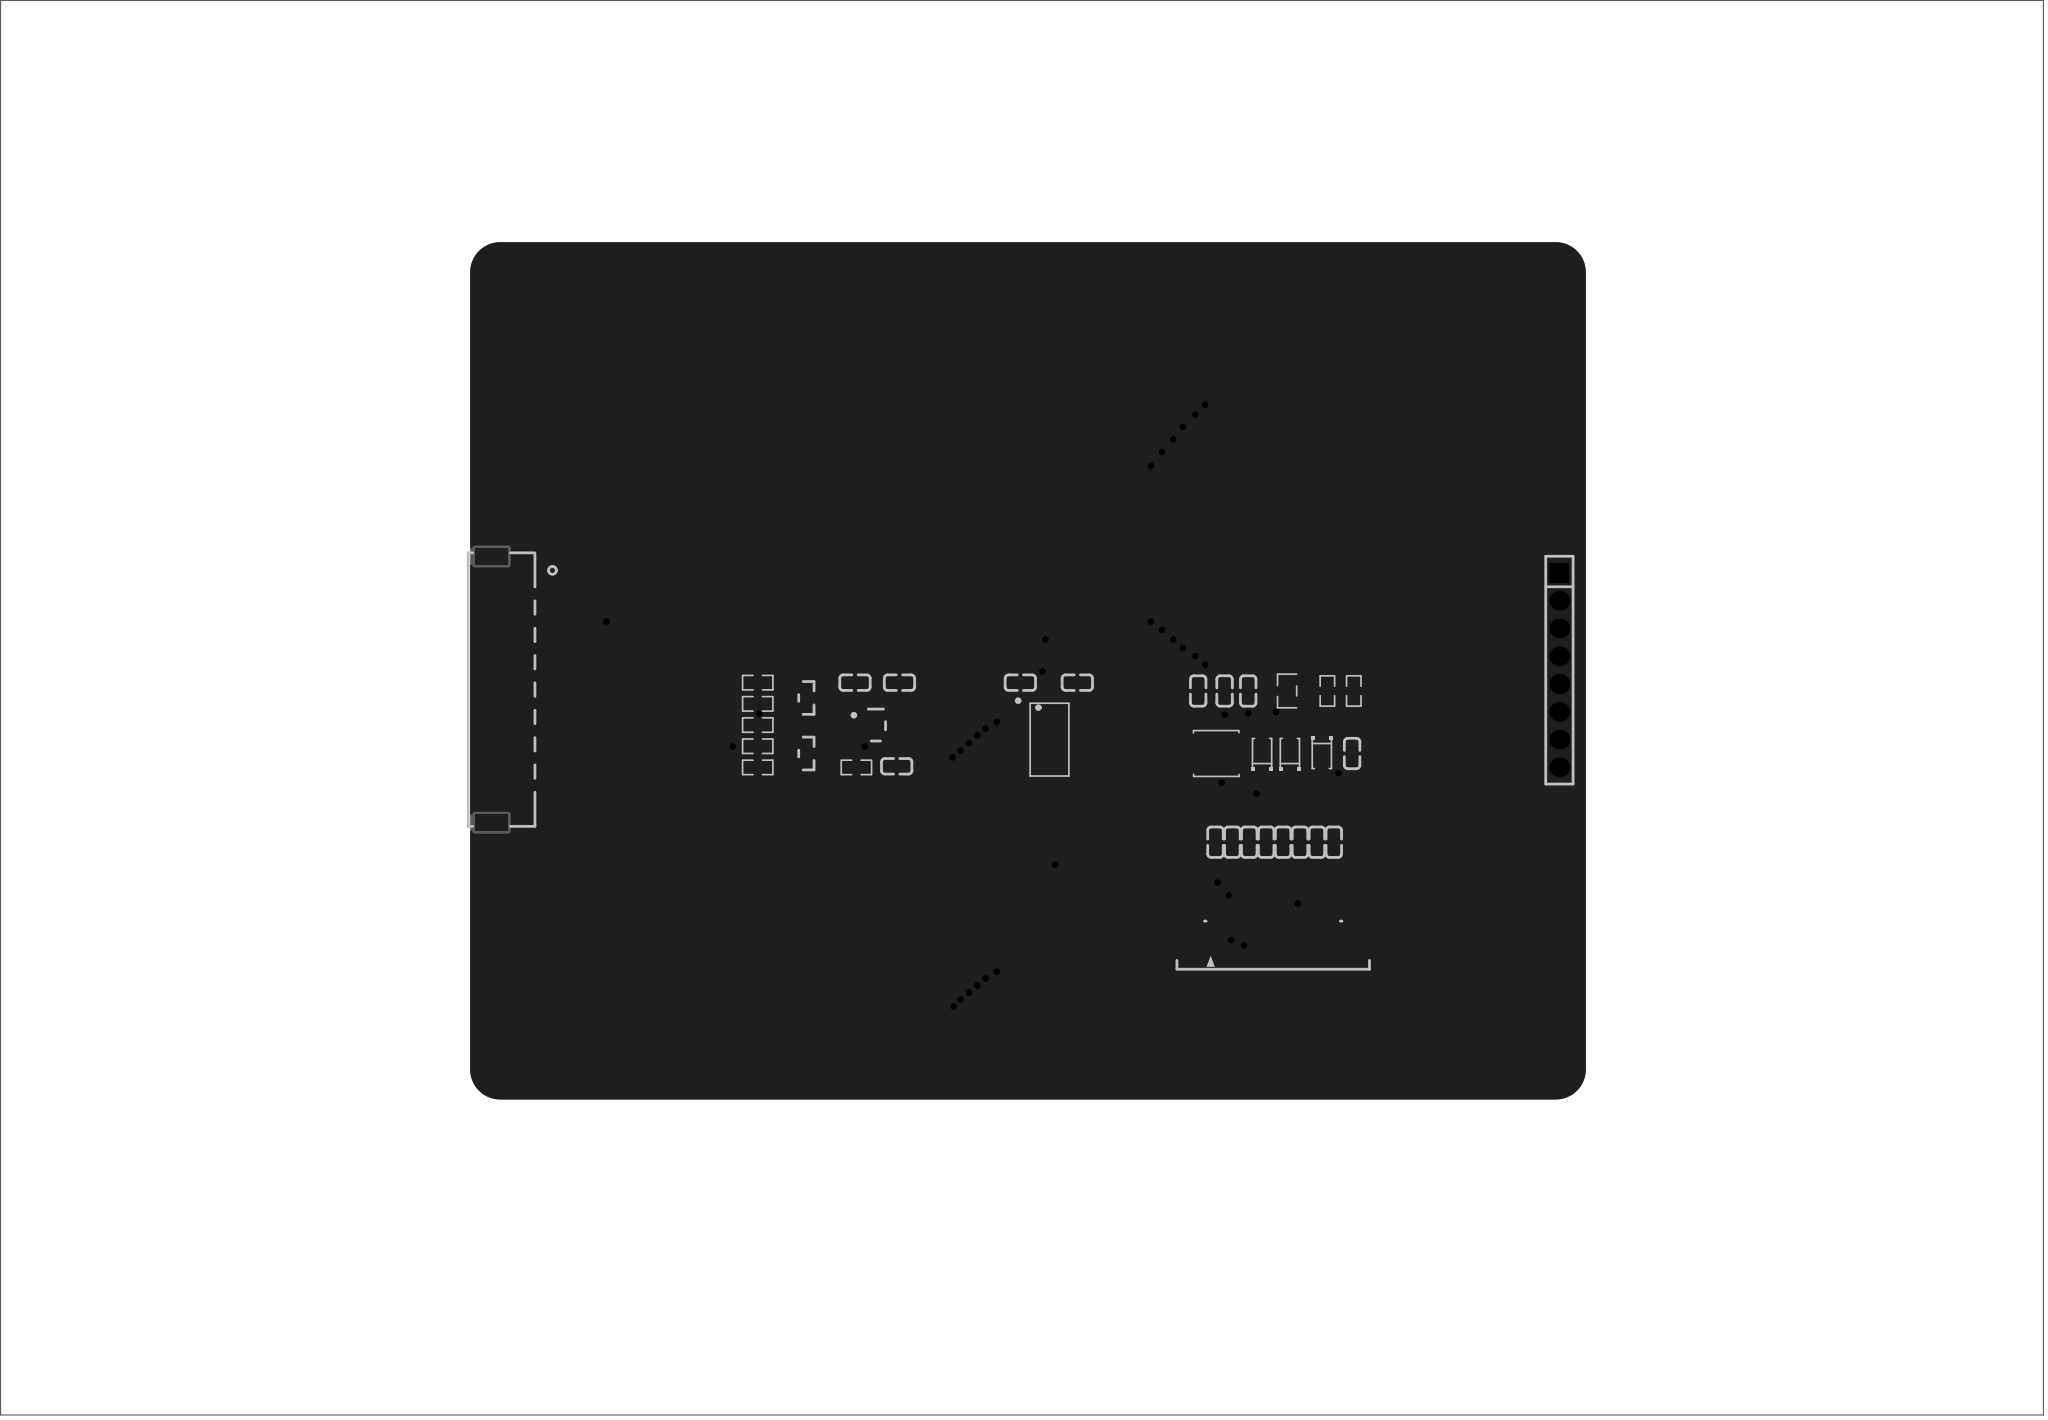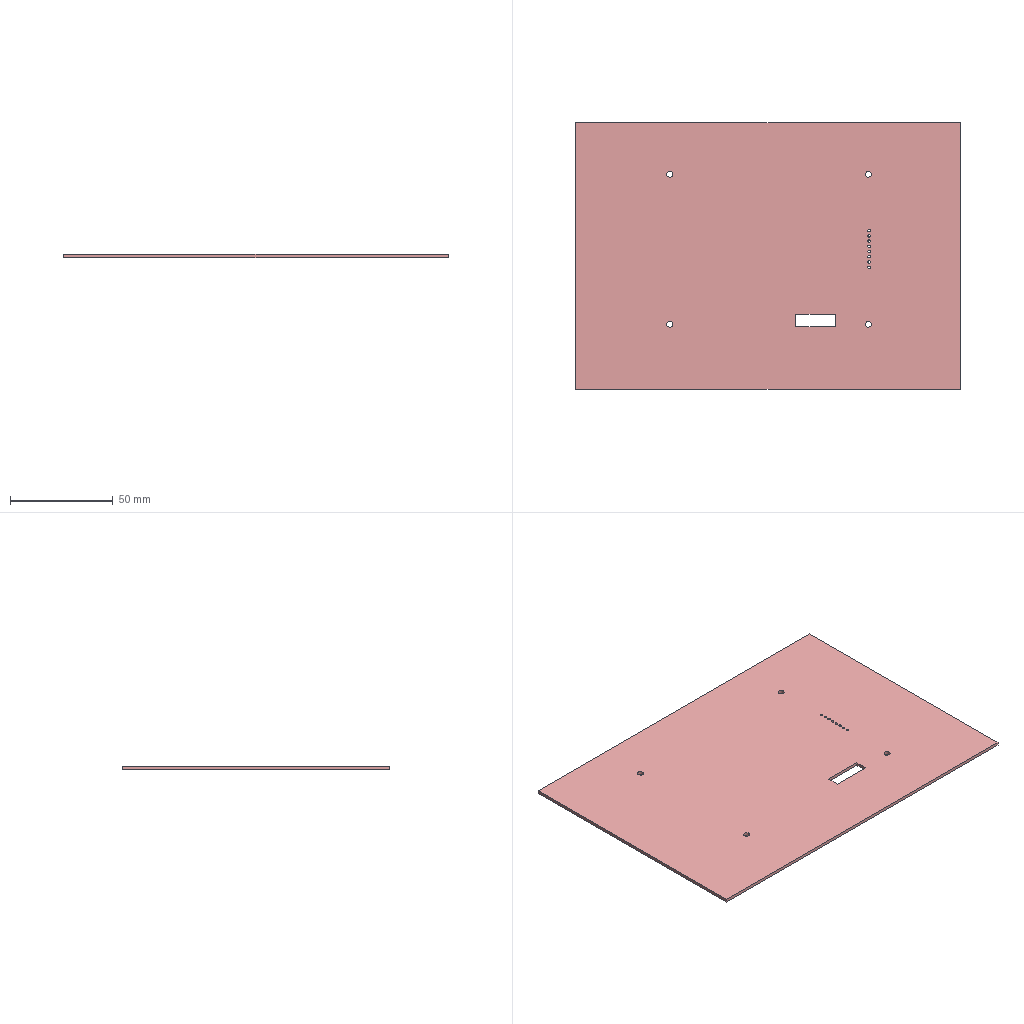Circuit board layout | Altium Designer | box 186.7 x 129.3 x 1.6 mm
Layer stack:
# Altium Designer layer stack of  (unit mm; dielectric type: 0 none, 1 core, 2 prepreg, 3 surface material)
index,name,kind,layer,copper_thickness_mm,dielectric_type,dielectric_thickness_mm,dielectric_material,dielectric_constant
0,Top Paste Mask Layer,other,,,,,,
1,Top Silkscreen Layer,other,,,,,,
2,Top Solder Mask Layer,dielectric,,,3,0.01,,3.3
3,Top Layer,copper,Top Layer,0.035,,,,
4,Dielectric1,dielectric,,,3,1.51,FR4,4.5
5,Bottom Layer,copper,Bottom Layer,0.035,,,,
6,Bottom Solder Mask Layer,dielectric,,,3,0.01,,3.3
7,Bottom Silkscreen Layer,other,,,,,,
8,Bottom Paste Mask Layer,other,,,,,,
# drill layer pairs: low layer,high layer
drill_pair,Top Layer,Bottom Layer
Part placement:
Designator,Comment,Layer,Footprint,Center-X(mm),Center-Y(mm),Rotation
Q1,BSS138LT1G,TopLayer,SOT-23-3_L2.9-W1.6-P1.90-LS2.8-BR,187.452,136.026,0
C4,4.7uF,TopLayer,C0603,179.324,136.026,270
C3,4.7uF,TopLayer,C0603,183.896,136.026,90
C1,1uF,TopLayer,C0603,191.721,122.205,270
C2,1uF,TopLayer,C0603,190.176,122.205,270
C5,1uF,TopLayer,C0603,180.904,122.205,270
C6,1uF,TopLayer,C0603,188.631,122.205,270
C7,1uF,TopLayer,C0603,187.085,122.205,270
C8,1uF,TopLayer,C0603,185.54,122.205,270
C9,1uF,TopLayer,C0603,181.737,136.026,270
C10,1uF,TopLayer,C0603,183.994,122.205,270
C11,1uF,TopLayer,C0603,193.395,130.31,270
C12,1uF,TopLayer,C0603,182.449,122.205,270
C16,1uF,TopLayer,C0603,147.953,136.788,0
C17,22nF,TopLayer,C0603,151.765,129.141,0
C13,100nF,TopLayer,C0603,152.019,136.788,180
C15,100nF,TopLayer,C0603,163.068,136.788,0
C14,100nF,TopLayer,C0603,168.275,136.788,0
D3,MBR0530,TopLayer,SOD-123FL_L2.7-W1.8-LS3.7-RD,185.166,130.31,90
D2,MBR0530,TopLayer,SOD-123FL_L2.7-W1.8-LS3.7-RD,190.627,130.31,270
D1,MBR0530,TopLayer,SOD-123FL_L2.7-W1.8-LS3.7-RD,187.706,130.31,90
J1,,TopLayer,HDR-TH_3P-P2.54-V-F,166.376,122.056,0
P1,,TopLayer,HDR-TH_8P-P2.54-V-F-1,212.344,137.931,270
L1,GCNR4018,TopLayer,IND-SMD_L4.0-W4.0,180.975,130.311,0
Q31,SI2301CDS-T1-E3,TopLayer,SOT-23_L2.9-W1.3-P1.90-LS2.4-BR,143.51,130.311,180
Q32,,TopLayer,S8050_SOT-23,143.51,135.391,180
R2,10K,TopLayer,R0603,193.548,136.026,270
R1,10K,TopLayer,R0603,191.135,136.026,90
R33,100K,TopLayer,R0603,139.065,129.041,180
R35,1K,TopLayer,R0603,139.065,134.851,0
R36,1K,TopLayer,R0603,139.065,132.914,0
R37,47K,TopLayer,R0603,139.065,130.977,0
R34,47K,TopLayer,R0603,139.065,136.788,0
R3,100K,TopLayer,R0603,148.082,129.041,0
J3,FPC0.5-24P/top-entry pull-out,TopLayer,FPC-SMD_24P-P0.50_SHOU-HAN_CTSJ-H2.0,186.182,114.182,0
U2,RT9193-33GB-MS,TopLayer,SOT-23-5_L2.9-W1.6-P0.95-LS2.8-BR,149.86,132.851,180
U1,TXB0108PWR,TopLayer,TSSOP-20_L6.5-W4.4-P0.65-LS6.4-BL,165.735,131.581,270
U3,XH2.54-LS-8P,TopLayer,CONN-SMD_XH2.54-LS-8P,116.713,136.153,270
Pad and via stacks:
# Altium Designer via and pad stacks of  (unit mm). Each distinct definition once, with the count of objects using it.
# via: kind,start_layer,end_layer,hole_mm,diameter_mm,mode(0 simple;1 top-mid-bottom;2 full stack),diameter_per_layer,count,example_net
# pad: kind,layer,hole_mm,hole_type(0 round;1 square;2 slot),plating,top_size,top_shape(1 round;2 rect;3 octagon;9 rounded rect),mid_size,bottom_size,mode,footprint,size_per_layer,count,example
pad,Top Layer,0,0,plated,1.07x0.6,2,1.07x0.6,1.07x0.6,0,SOT-23-3_L2.9-W1.6-P1.90-LS2.8-BR,,3,Q1.1
pad,Top Layer,0,0,plated,0.8x0.9,2,0.8x0.9,0.8x0.9,0,C0603,,34,C4.2
pad,Top Layer,0,0,plated,1.2x1.15,2,1.2x1.15,1.2x1.15,0,SOD-123FL_L2.7-W1.8-LS3.7-RD,,6,D3.2
pad,Top Layer,0,0,plated,1.575x1.575,2,1.575x1.575,1.575x1.575,0,HDR-TH_3P-P2.54-V-F,,3,J1.3
pad,Top Layer,0,0,plated,1.6x3.5,2,1.6x3.5,1.6x3.5,0,IND-SMD_L4.0-W4.0,,2,L1.2
pad,Top Layer,0,0,plated,1x0.8,2,1x0.8,1x0.8,0,SOT-23_L2.9-W1.3-P1.90-LS2.4-BR,,3,Q31.2
pad,Top Layer,0,0,plated,1x0.8,2,1x0.8,1x0.8,0,S8050_SOT-23,,3,Q32.2
pad,Top Layer,0,0,plated,0.8065x0.864,2,0.8065x0.864,0.8065x0.864,0,R0603,,16,R2.2
pad,Top Layer,0,0,plated,0.3x1.8,2,0.3x1.8,0.3x1.8,0,FPC-SMD_24P-P0.50_SHOU-HAN_CTSJ-H2.0,,24,J3.24
pad,Top Layer,0,0,plated,3.2x2.5,2,3.2x2.5,3.2x2.5,0,FPC-SMD_24P-P0.50_SHOU-HAN_CTSJ-H2.0,,2,J3.25
pad,Top Layer,0,0,plated,0.6x1,2,0.6x1,0.6x1,0,SOT-23-5_L2.9-W1.6-P0.95-LS2.8-BR,,5,U2.2
pad,Top Layer,0,0,plated,0.364x1.742,1,0.364x1.742,0.364x1.742,0,TSSOP-20_L6.5-W4.4-P0.65-LS6.4-BL,,20,U1.1
pad,Top Layer,0,0,plated,0.8x6.5,2,0.8x6.5,0.8x6.5,0,CONN-SMD_XH2.54-LS-8P,,8,U3.8
pad,Top Layer,0,0,plated,1.5x3,2,1.5x3,1.5x3,0,CONN-SMD_XH2.54-LS-8P,,2,U3.9
pad,Multi-Layer,1.2,0,plated,1.8x1.8,2,1.8x1.8,1.8x1.8,0,HDR-TH_8P-P2.54-V-F-1,,1,P1.1
pad,Multi-Layer,1.2,0,plated,1.8x1.8,1,1.8x1.8,1.8x1.8,0,HDR-TH_8P-P2.54-V-F-1,,7,P1.2
via,Top Layer,Bottom Layer,0.3048,0.61,0,,42,DIN'
Copper pours:
name,layer,net,type(0 solid;1 hatched;2 none)
Top Layer-GND,Top Layer,GND,0
Bottom Layer-GND,Bottom Layer,GND,0